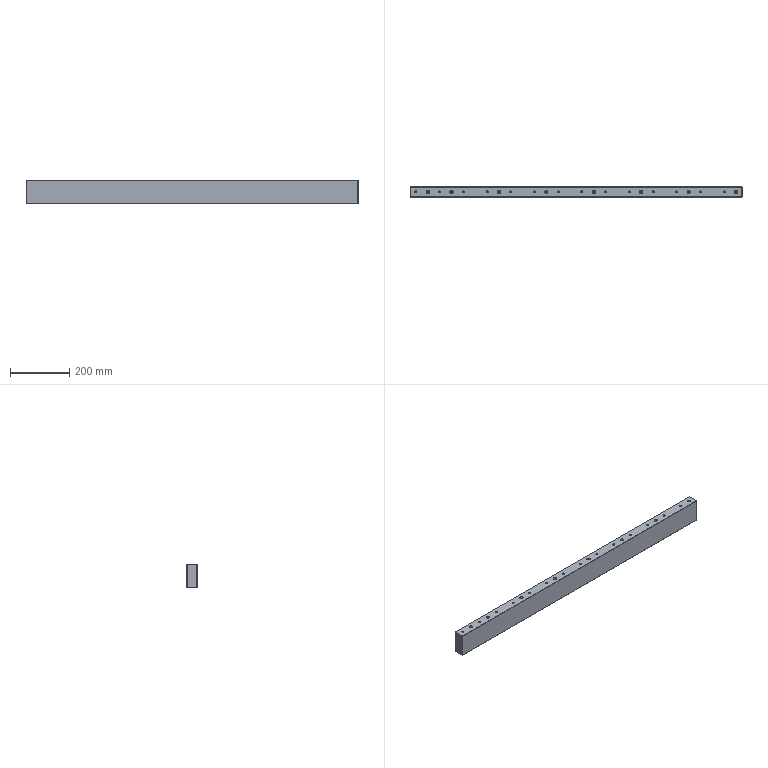Part | STEP file | TJ-DHQM-004-005 | 1 solid | 116 faces | box 1120 x 35 x 80 mm | volume 3082362 mm3 | cylinder 60 | cone 28 | plane 28 | commonest cylinder face diameters 6.8 x28 6.6 x16 11 x16